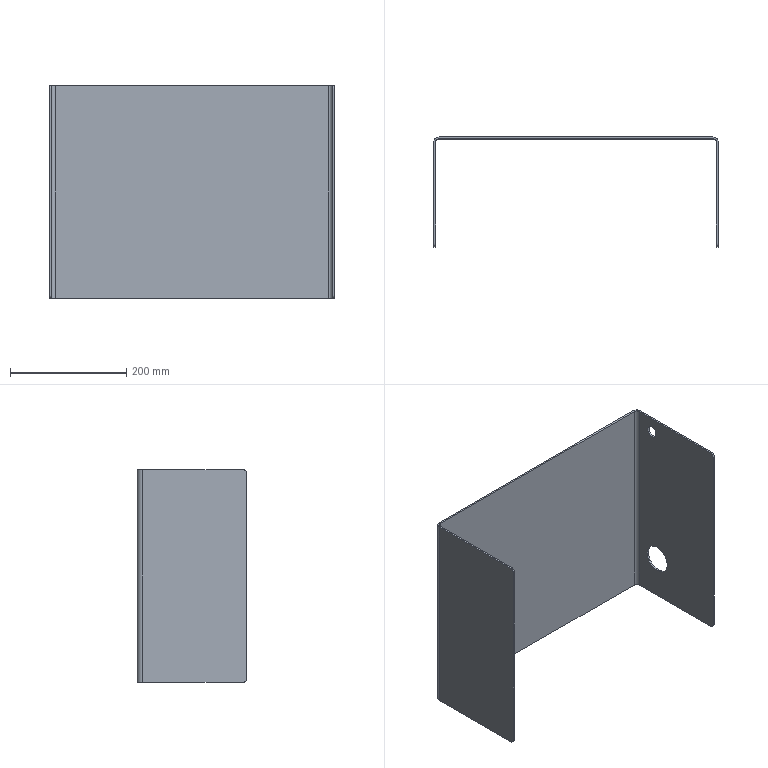Part | SolidWorks | features ICE 3, Cut 1, FlatPattern 1, SMBaseFlange 1, SheetMetal 1 | 1 solid | 30 faces | box 490 x 189 x 366 mm | volume 932829 mm3 | plane 18 | cylinder 12 | commonest cylinder face diameters 12 x6 18 x2 20 x2 48.5 x2
STEP:
#1=CARTESIAN_POINT('',(484.,-37.,349.));
#2=VERTEX_POINT('',#1);
#3=CARTESIAN_POINT('',(484.,-37.,329.));
#4=VERTEX_POINT('',#3);
#5=CARTESIAN_POINT('',(484.,-37.,339.));
#6=DIRECTION('',(1.,0.,0.));
#7=DIRECTION('',(0.,0.,-1.));
#8=AXIS2_PLACEMENT_3D('',#5,#6,#7);
#9=CIRCLE('',#8,10.);
#10=EDGE_CURVE('',#2,#4,#9,.T.);
#11=ORIENTED_EDGE('',*,*,#10,.F.);
#12=CARTESIAN_POINT('',(487.,-37.,349.));
#13=VERTEX_POINT('',#12);
#14=CARTESIAN_POINT('',(477.,-37.,349.));
#15=DIRECTION('',(1.,0.,0.));
#16=VECTOR('',#15,1000.);
#17=LINE('',#14,#16);
#18=EDGE_CURVE('',#2,#13,#17,.T.);
#19=ORIENTED_EDGE('',*,*,#18,.T.);
#20=CARTESIAN_POINT('',(487.,-37.,329.));
#21=VERTEX_POINT('',#20);
#22=CARTESIAN_POINT('',(487.,-37.,339.));
#23=DIRECTION('',(1.,0.,0.));
#24=DIRECTION('',(0.,0.,-1.));
#25=AXIS2_PLACEMENT_3D('',#22,#23,#24);
#26=CIRCLE('',#25,10.);
#27=EDGE_CURVE('',#13,#21,#26,.T.);
#28=ORIENTED_EDGE('',*,*,#27,.T.);
#29=CARTESIAN_POINT('',(477.,-37.,329.));
#30=DIRECTION('',(1.,0.,0.));
#31=VECTOR('',#30,1000.);
#32=LINE('',#29,#31);
#33=EDGE_CURVE('',#4,#21,#32,.T.);
#34=ORIENTED_EDGE('',*,*,#33,.F.);
#35=EDGE_LOOP('',(#11,#19,#28,#34));
#36=FACE_OUTER_BOUND('',#35,.T.);
#37=CARTESIAN_POINT('',(477.,-37.,339.));
#38=DIRECTION('',(1.,0.,0.));
#39=DIRECTION('',(0.,0.,-1.));
#40=AXIS2_PLACEMENT_3D('',#37,#38,#39);
#41=CYLINDRICAL_SURFACE('',#40,10.);
#42=ADVANCED_FACE('',(#36),#41,.F.);
#43=CARTESIAN_POINT('',(484.,-50.,101.25));
#44=VERTEX_POINT('',#43);
#45=CARTESIAN_POINT('',(484.,-50.,52.75));
#46=VERTEX_POINT('',#45);
#47=CARTESIAN_POINT('',(484.,-50.,77.));
#48=DIRECTION('',(1.,0.,0.));
#49=DIRECTION('',(0.,0.,-1.));
#50=AXIS2_PLACEMENT_3D('',#47,#48,#49);
#51=CIRCLE('',#50,24.25);
#52=EDGE_CURVE('',#44,#46,#51,.T.);
#53=ORIENTED_EDGE('',*,*,#52,.F.);
#54=CARTESIAN_POINT('',(487.,-50.,101.25));
#55=VERTEX_POINT('',#54);
#56=CARTESIAN_POINT('',(477.,-50.,101.25));
#57=DIRECTION('',(1.,0.,0.));
#58=VECTOR('',#57,1000.);
#59=LINE('',#56,#58);
#60=EDGE_CURVE('',#44,#55,#59,.T.);
#61=ORIENTED_EDGE('',*,*,#60,.T.);
#62=CARTESIAN_POINT('',(487.,-50.,52.75));
#63=VERTEX_POINT('',#62);
#64=CARTESIAN_POINT('',(487.,-50.,77.));
#65=DIRECTION('',(1.,0.,0.));
#66=DIRECTION('',(0.,0.,-1.));
#67=AXIS2_PLACEMENT_3D('',#64,#65,#66);
#68=CIRCLE('',#67,24.25);
#69=EDGE_CURVE('',#55,#63,#68,.T.);
#70=ORIENTED_EDGE('',*,*,#69,.T.);
#71=CARTESIAN_POINT('',(477.,-50.,52.75));
#72=DIRECTION('',(1.,0.,0.));
#73=VECTOR('',#72,1000.);
#74=LINE('',#71,#73);
#75=EDGE_CURVE('',#46,#63,#74,.T.);
#76=ORIENTED_EDGE('',*,*,#75,.F.);
#77=EDGE_LOOP('',(#53,#61,#70,#76));
#78=FACE_OUTER_BOUND('',#77,.T.);
#79=CARTESIAN_POINT('',(477.,-50.,77.));
#80=DIRECTION('',(1.,0.,0.));
#81=DIRECTION('',(0.,0.,-1.));
#82=AXIS2_PLACEMENT_3D('',#79,#80,#81);
#83=CYLINDRICAL_SURFACE('',#82,24.25);
#84=ADVANCED_FACE('',(#78),#83,.F.);
#85=CARTESIAN_POINT('',(-3.,-180.,0.));
#86=VERTEX_POINT('',#85);
#87=CARTESIAN_POINT('',(-3.,-6.,0.));
#88=VERTEX_POINT('',#87);
#89=CARTESIAN_POINT('',(-3.,0.,0.));
#90=DIRECTION('',(0.,1.,0.));
#91=VECTOR('',#90,1000.);
#92=LINE('',#89,#91);
#93=EDGE_CURVE('',#86,#88,#92,.T.);
#94=ORIENTED_EDGE('',*,*,#93,.F.);
#95=CARTESIAN_POINT('',(-3.,-186.,6.));
#96=VERTEX_POINT('',#95);
#97=CARTESIAN_POINT('',(-3.,-180.,6.));
#98=DIRECTION('',(1.,0.,0.));
#99=DIRECTION('',(0.,-1.,0.));
#100=AXIS2_PLACEMENT_3D('',#97,#98,#99);
#101=CIRCLE('',#100,6.);
#102=EDGE_CURVE('',#96,#86,#101,.T.);
#103=ORIENTED_EDGE('',*,*,#102,.F.);
#104=CARTESIAN_POINT('',(-3.,-186.,360.));
#105=VERTEX_POINT('',#104);
#106=CARTESIAN_POINT('',(-3.,-186.,366.));
#107=DIRECTION('',(0.,0.,1.));
#108=VECTOR('',#107,1000.);
#109=LINE('',#106,#108);
#110=EDGE_CURVE('',#96,#105,#109,.T.);
#111=ORIENTED_EDGE('',*,*,#110,.T.);
#112=CARTESIAN_POINT('',(-3.,-180.,366.));
#113=VERTEX_POINT('',#112);
#114=CARTESIAN_POINT('',(-3.,-180.,360.));
#115=DIRECTION('',(1.,0.,0.));
#116=DIRECTION('',(0.,-1.,0.));
#117=AXIS2_PLACEMENT_3D('',#114,#115,#116);
#118=CIRCLE('',#117,6.);
#119=EDGE_CURVE('',#113,#105,#118,.T.);
#120=ORIENTED_EDGE('',*,*,#119,.F.);
#121=CARTESIAN_POINT('',(-3.,-6.,366.));
#122=VERTEX_POINT('',#121);
#123=CARTESIAN_POINT('',(-3.,0.,366.));
#124=DIRECTION('',(0.,1.,0.));
#125=VECTOR('',#124,1000.);
#126=LINE('',#123,#125);
#127=EDGE_CURVE('',#113,#122,#126,.T.);
#128=ORIENTED_EDGE('',*,*,#127,.T.);
#129=CARTESIAN_POINT('',(-3.,-6.,366.));
#130=DIRECTION('',(0.,0.,-1.));
#131=VECTOR('',#130,1000.);
#132=LINE('',#129,#131);
#133=EDGE_CURVE('',#122,#88,#132,.T.);
#134=ORIENTED_EDGE('',*,*,#133,.T.);
#135=EDGE_LOOP('',(#94,#103,#111,#120,#128,#134));
#136=FACE_OUTER_BOUND('',#135,.T.);
#137=CARTESIAN_POINT('',(-3.,0.,366.));
#138=DIRECTION('',(-1.,0.,0.));
#139=DIRECTION('',(0.,-1.,0.));
#140=AXIS2_PLACEMENT_3D('',#137,#138,#139);
#141=PLANE('',#140);
#142=ADVANCED_FACE('',(#136),#141,.T.);
#143=CARTESIAN_POINT('',(0.,-186.,6.));
#144=VERTEX_POINT('',#143);
#145=CARTESIAN_POINT('',(0.,-180.,0.));
#146=VERTEX_POINT('',#145);
#147=CARTESIAN_POINT('',(0.,-180.,6.));
#148=DIRECTION('',(1.,0.,0.));
#149=DIRECTION('',(0.,-1.,0.));
#150=AXIS2_PLACEMENT_3D('',#147,#148,#149);
#151=CIRCLE('',#150,6.);
#152=EDGE_CURVE('',#144,#146,#151,.T.);
#153=ORIENTED_EDGE('',*,*,#152,.T.);
#154=CARTESIAN_POINT('',(0.,-6.,0.));
#155=VERTEX_POINT('',#154);
#156=CARTESIAN_POINT('',(0.,0.,0.));
#157=DIRECTION('',(0.,1.,0.));
#158=VECTOR('',#157,1000.);
#159=LINE('',#156,#158);
#160=EDGE_CURVE('',#146,#155,#159,.T.);
#161=ORIENTED_EDGE('',*,*,#160,.T.);
#162=CARTESIAN_POINT('',(0.,-6.,366.));
#163=VERTEX_POINT('',#162);
#164=CARTESIAN_POINT('',(0.,-6.,366.));
#165=DIRECTION('',(0.,0.,-1.));
#166=VECTOR('',#165,1000.);
#167=LINE('',#164,#166);
#168=EDGE_CURVE('',#163,#155,#167,.T.);
#169=ORIENTED_EDGE('',*,*,#168,.F.);
#170=CARTESIAN_POINT('',(0.,-180.,366.));
#171=VERTEX_POINT('',#170);
#172=CARTESIAN_POINT('',(0.,0.,366.));
#173=DIRECTION('',(0.,1.,0.));
#174=VECTOR('',#173,1000.);
#175=LINE('',#172,#174);
#176=EDGE_CURVE('',#171,#163,#175,.T.);
#177=ORIENTED_EDGE('',*,*,#176,.F.);
#178=CARTESIAN_POINT('',(0.,-186.,360.));
#179=VERTEX_POINT('',#178);
#180=CARTESIAN_POINT('',(0.,-180.,360.));
#181=DIRECTION('',(1.,0.,0.));
#182=DIRECTION('',(0.,-1.,0.));
#183=AXIS2_PLACEMENT_3D('',#180,#181,#182);
#184=CIRCLE('',#183,6.);
#185=EDGE_CURVE('',#171,#179,#184,.T.);
#186=ORIENTED_EDGE('',*,*,#185,.T.);
#187=CARTESIAN_POINT('',(0.,-186.,366.));
#188=DIRECTION('',(0.,0.,-1.));
#189=VECTOR('',#188,1000.);
#190=LINE('',#187,#189);
#191=EDGE_CURVE('',#179,#144,#190,.T.);
#192=ORIENTED_EDGE('',*,*,#191,.T.);
#193=EDGE_LOOP('',(#153,#161,#169,#177,#186,#192));
#194=FACE_OUTER_BOUND('',#193,.T.);
#195=CARTESIAN_POINT('',(0.,0.,366.));
#196=DIRECTION('',(-1.,0.,0.));
#197=DIRECTION('',(0.,-1.,0.));
#198=AXIS2_PLACEMENT_3D('',#195,#196,#197);
#199=PLANE('',#198);
#200=ADVANCED_FACE('',(#194),#199,.F.);
#201=CARTESIAN_POINT('',(0.,-186.,6.));
#202=DIRECTION('',(-1.,0.,0.));
#203=VECTOR('',#202,1000.);
#204=LINE('',#201,#203);
#205=EDGE_CURVE('',#144,#96,#204,.T.);
#206=ORIENTED_EDGE('',*,*,#205,.F.);
#207=ORIENTED_EDGE('',*,*,#191,.F.);
#208=CARTESIAN_POINT('',(0.,-186.,360.));
#209=DIRECTION('',(-1.,0.,0.));
#210=VECTOR('',#209,1000.);
#211=LINE('',#208,#210);
#212=EDGE_CURVE('',#179,#105,#211,.T.);
#213=ORIENTED_EDGE('',*,*,#212,.T.);
#214=ORIENTED_EDGE('',*,*,#110,.F.);
#215=EDGE_LOOP('',(#206,#207,#213,#214));
#216=FACE_OUTER_BOUND('',#215,.T.);
#217=CARTESIAN_POINT('',(-3.,-186.,366.));
#218=DIRECTION('',(0.,1.,0.));
#219=DIRECTION('',(0.,0.,1.));
#220=AXIS2_PLACEMENT_3D('',#217,#218,#219);
#221=PLANE('',#220);
#222=ADVANCED_FACE('',(#216),#221,.F.);
#223=CARTESIAN_POINT('',(484.,-37.,339.));
#224=DIRECTION('',(1.,0.,0.));
#225=DIRECTION('',(0.,0.,-1.));
#226=AXIS2_PLACEMENT_3D('',#223,#224,#225);
#227=CIRCLE('',#226,10.);
#228=EDGE_CURVE('',#4,#2,#227,.T.);
#229=ORIENTED_EDGE('',*,*,#228,.T.);
#230=ORIENTED_EDGE('',*,*,#10,.T.);
#231=EDGE_LOOP('',(#229,#230));
#232=FACE_BOUND('',#231,.T.);
#233=CARTESIAN_POINT('',(484.,-50.,77.));
#234=DIRECTION('',(1.,0.,0.));
#235=DIRECTION('',(0.,0.,-1.));
#236=AXIS2_PLACEMENT_3D('',#233,#234,#235);
#237=CIRCLE('',#236,24.25);
#238=EDGE_CURVE('',#46,#44,#237,.T.);
#239=ORIENTED_EDGE('',*,*,#238,.T.);
#240=ORIENTED_EDGE('',*,*,#52,.T.);
#241=EDGE_LOOP('',(#239,#240));
#242=FACE_BOUND('',#241,.T.);
#243=CARTESIAN_POINT('',(484.,-186.,360.));
#244=VERTEX_POINT('',#243);
#245=CARTESIAN_POINT('',(484.,-180.,366.));
#246=VERTEX_POINT('',#245);
#247=CARTESIAN_POINT('',(484.,-180.,360.));
#248=DIRECTION('',(-1.,0.,0.));
#249=DIRECTION('',(0.,0.,-1.));
#250=AXIS2_PLACEMENT_3D('',#247,#248,#249);
#251=CIRCLE('',#250,6.);
#252=EDGE_CURVE('',#244,#246,#251,.T.);
#253=ORIENTED_EDGE('',*,*,#252,.T.);
#254=CARTESIAN_POINT('',(484.,-6.,366.));
#255=VERTEX_POINT('',#254);
#256=CARTESIAN_POINT('',(484.,0.,366.));
#257=DIRECTION('',(0.,-1.,0.));
#258=VECTOR('',#257,1000.);
#259=LINE('',#256,#258);
#260=EDGE_CURVE('',#255,#246,#259,.T.);
#261=ORIENTED_EDGE('',*,*,#260,.F.);
#262=CARTESIAN_POINT('',(484.,-6.,0.));
#263=VERTEX_POINT('',#262);
#264=CARTESIAN_POINT('',(484.,-6.,366.));
#265=DIRECTION('',(0.,0.,-1.));
#266=VECTOR('',#265,1000.);
#267=LINE('',#264,#266);
#268=EDGE_CURVE('',#255,#263,#267,.T.);
#269=ORIENTED_EDGE('',*,*,#268,.T.);
#270=CARTESIAN_POINT('',(484.,-180.,0.));
#271=VERTEX_POINT('',#270);
#272=CARTESIAN_POINT('',(484.,0.,0.));
#273=DIRECTION('',(0.,-1.,0.));
#274=VECTOR('',#273,1000.);
#275=LINE('',#272,#274);
#276=EDGE_CURVE('',#263,#271,#275,.T.);
#277=ORIENTED_EDGE('',*,*,#276,.T.);
#278=CARTESIAN_POINT('',(484.,-186.,6.));
#279=VERTEX_POINT('',#278);
#280=CARTESIAN_POINT('',(484.,-180.,6.));
#281=DIRECTION('',(-1.,0.,0.));
#282=DIRECTION('',(0.,0.,-1.));
#283=AXIS2_PLACEMENT_3D('',#280,#281,#282);
#284=CIRCLE('',#283,6.);
#285=EDGE_CURVE('',#271,#279,#284,.T.);
#286=ORIENTED_EDGE('',*,*,#285,.T.);
#287=CARTESIAN_POINT('',(484.,-186.,366.));
#288=DIRECTION('',(0.,0.,1.));
#289=VECTOR('',#288,1000.);
#290=LINE('',#287,#289);
#291=EDGE_CURVE('',#279,#244,#290,.T.);
#292=ORIENTED_EDGE('',*,*,#291,.T.);
#293=EDGE_LOOP('',(#253,#261,#269,#277,#286,#292));
#294=FACE_OUTER_BOUND('',#293,.T.);
#295=CARTESIAN_POINT('',(484.,0.,366.));
#296=DIRECTION('',(1.,0.,0.));
#297=DIRECTION('',(0.,0.,-1.));
#298=AXIS2_PLACEMENT_3D('',#295,#296,#297);
#299=PLANE('',#298);
#300=ADVANCED_FACE('',(#232,#242,#294),#299,.F.);
#301=CARTESIAN_POINT('',(487.,-37.,339.));
#302=DIRECTION('',(1.,0.,0.));
#303=DIRECTION('',(0.,0.,-1.));
#304=AXIS2_PLACEMENT_3D('',#301,#302,#303);
#305=CIRCLE('',#304,10.);
#306=EDGE_CURVE('',#21,#13,#305,.T.);
#307=ORIENTED_EDGE('',*,*,#306,.F.);
#308=ORIENTED_EDGE('',*,*,#27,.F.);
#309=EDGE_LOOP('',(#307,#308));
#310=FACE_BOUND('',#309,.T.);
#311=CARTESIAN_POINT('',(487.,-50.,77.));
#312=DIRECTION('',(1.,0.,0.));
#313=DIRECTION('',(0.,0.,-1.));
#314=AXIS2_PLACEMENT_3D('',#311,#312,#313);
#315=CIRCLE('',#314,24.25);
#316=EDGE_CURVE('',#63,#55,#315,.T.);
#317=ORIENTED_EDGE('',*,*,#316,.F.);
#318=ORIENTED_EDGE('',*,*,#69,.F.);
#319=EDGE_LOOP('',(#317,#318));
#320=FACE_BOUND('',#319,.T.);
#321=CARTESIAN_POINT('',(487.,-6.,366.));
#322=VERTEX_POINT('',#321);
#323=CARTESIAN_POINT('',(487.,-180.,366.));
#324=VERTEX_POINT('',#323);
#325=CARTESIAN_POINT('',(487.,0.,366.));
#326=DIRECTION('',(0.,-1.,0.));
#327=VECTOR('',#326,1000.);
#328=LINE('',#325,#327);
#329=EDGE_CURVE('',#322,#324,#328,.T.);
#330=ORIENTED_EDGE('',*,*,#329,.T.);
#331=CARTESIAN_POINT('',(487.,-186.,360.));
#332=VERTEX_POINT('',#331);
#333=CARTESIAN_POINT('',(487.,-180.,360.));
#334=DIRECTION('',(-1.,0.,0.));
#335=DIRECTION('',(0.,0.,-1.));
#336=AXIS2_PLACEMENT_3D('',#333,#334,#335);
#337=CIRCLE('',#336,6.);
#338=EDGE_CURVE('',#332,#324,#337,.T.);
#339=ORIENTED_EDGE('',*,*,#338,.F.);
#340=CARTESIAN_POINT('',(487.,-186.,6.));
#341=VERTEX_POINT('',#340);
#342=CARTESIAN_POINT('',(487.,-186.,366.));
#343=DIRECTION('',(0.,0.,1.));
#344=VECTOR('',#343,1000.);
#345=LINE('',#342,#344);
#346=EDGE_CURVE('',#341,#332,#345,.T.);
#347=ORIENTED_EDGE('',*,*,#346,.F.);
#348=CARTESIAN_POINT('',(487.,-180.,0.));
#349=VERTEX_POINT('',#348);
#350=CARTESIAN_POINT('',(487.,-180.,6.));
#351=DIRECTION('',(-1.,0.,0.));
#352=DIRECTION('',(0.,0.,-1.));
#353=AXIS2_PLACEMENT_3D('',#350,#351,#352);
#354=CIRCLE('',#353,6.);
#355=EDGE_CURVE('',#349,#341,#354,.T.);
#356=ORIENTED_EDGE('',*,*,#355,.F.);
#357=CARTESIAN_POINT('',(487.,-6.,0.));
#358=VERTEX_POINT('',#357);
#359=CARTESIAN_POINT('',(487.,0.,0.));
#360=DIRECTION('',(0.,-1.,0.));
#361=VECTOR('',#360,1000.);
#362=LINE('',#359,#361);
#363=EDGE_CURVE('',#358,#349,#362,.T.);
#364=ORIENTED_EDGE('',*,*,#363,.F.);
#365=CARTESIAN_POINT('',(487.,-6.,366.));
#366=DIRECTION('',(0.,0.,-1.));
#367=VECTOR('',#366,1000.);
#368=LINE('',#365,#367);
#369=EDGE_CURVE('',#322,#358,#368,.T.);
#370=ORIENTED_EDGE('',*,*,#369,.F.);
#371=EDGE_LOOP('',(#330,#339,#347,#356,#364,#370));
#372=FACE_OUTER_BOUND('',#371,.T.);
#373=CARTESIAN_POINT('',(487.,0.,366.));
#374=DIRECTION('',(1.,0.,0.));
#375=DIRECTION('',(0.,0.,-1.));
#376=AXIS2_PLACEMENT_3D('',#373,#374,#375);
#377=PLANE('',#376);
#378=ADVANCED_FACE('',(#310,#320,#372),#377,.T.);
#379=ORIENTED_EDGE('',*,*,#260,.T.);
#380=CARTESIAN_POINT('',(484.,-180.,366.));
#381=DIRECTION('',(1.,0.,0.));
#382=VECTOR('',#381,1000.);
#383=LINE('',#380,#382);
#384=EDGE_CURVE('',#246,#324,#383,.T.);
#385=ORIENTED_EDGE('',*,*,#384,.T.);
#386=ORIENTED_EDGE('',*,*,#329,.F.);
#387=CARTESIAN_POINT('',(487.,-6.,366.));
#388=DIRECTION('',(-1.,0.,0.));
#389=VECTOR('',#388,1000.);
#390=LINE('',#387,#389);
#391=EDGE_CURVE('',#322,#255,#390,.T.);
#392=ORIENTED_EDGE('',*,*,#391,.T.);
#393=EDGE_LOOP('',(#379,#385,#386,#392));
#394=FACE_OUTER_BOUND('',#393,.T.);
#395=CARTESIAN_POINT('',(478.,-6.,366.));
#396=DIRECTION('',(0.,0.,1.));
#397=DIRECTION('',(1.,0.,0.));
#398=AXIS2_PLACEMENT_3D('',#395,#396,#397);
#399=PLANE('',#398);
#400=ADVANCED_FACE('',(#394),#399,.T.);
#401=CARTESIAN_POINT('',(484.,-186.,360.));
#402=DIRECTION('',(1.,0.,0.));
#403=VECTOR('',#402,1000.);
#404=LINE('',#401,#403);
#405=EDGE_CURVE('',#244,#332,#404,.T.);
#406=ORIENTED_EDGE('',*,*,#405,.F.);
#407=ORIENTED_EDGE('',*,*,#291,.F.);
#408=CARTESIAN_POINT('',(484.,-186.,6.));
#409=DIRECTION('',(1.,0.,0.));
#410=VECTOR('',#409,1000.);
#411=LINE('',#408,#410);
#412=EDGE_CURVE('',#279,#341,#411,.T.);
#413=ORIENTED_EDGE('',*,*,#412,.T.);
#414=ORIENTED_EDGE('',*,*,#346,.T.);
#415=EDGE_LOOP('',(#406,#407,#413,#414));
#416=FACE_OUTER_BOUND('',#415,.T.);
#417=CARTESIAN_POINT('',(-3.,-186.,366.));
#418=DIRECTION('',(0.,1.,0.));
#419=DIRECTION('',(0.,0.,1.));
#420=AXIS2_PLACEMENT_3D('',#417,#418,#419);
#421=PLANE('',#420);
#422=ADVANCED_FACE('',(#416),#421,.F.);
#423=CARTESIAN_POINT('',(0.,-6.,366.));
#424=DIRECTION('',(-1.,0.,0.));
#425=VECTOR('',#424,1000.);
#426=LINE('',#423,#425);
#427=EDGE_CURVE('',#163,#122,#426,.T.);
#428=ORIENTED_EDGE('',*,*,#427,.F.);
#429=CARTESIAN_POINT('',(6.,0.,366.));
#430=VERTEX_POINT('',#429);
#431=CARTESIAN_POINT('',(6.,-6.,366.));
#432=DIRECTION('',(0.,0.,-1.));
#433=DIRECTION('',(1.,0.,0.));
#434=AXIS2_PLACEMENT_3D('',#431,#432,#433);
#435=CIRCLE('',#434,6.);
#436=EDGE_CURVE('',#163,#430,#435,.T.);
#437=ORIENTED_EDGE('',*,*,#436,.T.);
#438=CARTESIAN_POINT('',(6.,3.,366.));
#439=VERTEX_POINT('',#438);
#440=CARTESIAN_POINT('',(6.,3.,366.));
#441=DIRECTION('',(0.,-1.,0.));
#442=VECTOR('',#441,1000.);
#443=LINE('',#440,#442);
#444=EDGE_CURVE('',#439,#430,#443,.T.);
#445=ORIENTED_EDGE('',*,*,#444,.F.);
#446=CARTESIAN_POINT('',(6.,-6.,366.));
#447=DIRECTION('',(0.,0.,-1.));
#448=DIRECTION('',(1.,0.,0.));
#449=AXIS2_PLACEMENT_3D('',#446,#447,#448);
#450=CIRCLE('',#449,9.);
#451=EDGE_CURVE('',#122,#439,#450,.T.);
#452=ORIENTED_EDGE('',*,*,#451,.F.);
#453=EDGE_LOOP('',(#428,#437,#445,#452));
#454=FACE_OUTER_BOUND('',#453,.T.);
#455=CARTESIAN_POINT('',(0.,-6.,366.));
#456=DIRECTION('',(0.,0.,1.));
#457=DIRECTION('',(1.,0.,0.));
#458=AXIS2_PLACEMENT_3D('',#455,#456,#457);
#459=PLANE('',#458);
#460=ADVANCED_FACE('',(#454),#459,.T.);
#461=CARTESIAN_POINT('',(0.,-180.,366.));
#462=DIRECTION('',(-1.,0.,0.));
#463=VECTOR('',#462,1000.);
#464=LINE('',#461,#463);
#465=EDGE_CURVE('',#171,#113,#464,.T.);
#466=ORIENTED_EDGE('',*,*,#465,.F.);
#467=ORIENTED_EDGE('',*,*,#176,.T.);
#468=ORIENTED_EDGE('',*,*,#427,.T.);
#469=ORIENTED_EDGE('',*,*,#127,.F.);
#470=EDGE_LOOP('',(#466,#467,#468,#469));
#471=FACE_OUTER_BOUND('',#470,.T.);
#472=CARTESIAN_POINT('',(6.,3.,366.));
#473=DIRECTION('',(0.,0.,1.));
#474=DIRECTION('',(1.,0.,0.));
#475=AXIS2_PLACEMENT_3D('',#472,#473,#474);
#476=PLANE('',#475);
#477=ADVANCED_FACE('',(#471),#476,.T.);
#478=CARTESIAN_POINT('',(6.,0.,0.));
#479=VERTEX_POINT('',#478);
#480=CARTESIAN_POINT('',(6.,3.,0.));
#481=VERTEX_POINT('',#480);
#482=CARTESIAN_POINT('',(6.,0.,0.));
#483=DIRECTION('',(0.,1.,0.));
#484=VECTOR('',#483,1000.);
#485=LINE('',#482,#484);
#486=EDGE_CURVE('',#479,#481,#485,.T.);
#487=ORIENTED_EDGE('',*,*,#486,.F.);
#488=CARTESIAN_POINT('',(6.,-6.,0.));
#489=DIRECTION('',(0.,0.,-1.));
#490=DIRECTION('',(1.,0.,0.));
#491=AXIS2_PLACEMENT_3D('',#488,#489,#490);
#492=CIRCLE('',#491,6.);
#493=EDGE_CURVE('',#155,#479,#492,.T.);
#494=ORIENTED_EDGE('',*,*,#493,.F.);
#495=CARTESIAN_POINT('',(-3.,-6.,0.));
#496=DIRECTION('',(1.,0.,0.));
#497=VECTOR('',#496,1000.);
#498=LINE('',#495,#497);
#499=EDGE_CURVE('',#88,#155,#498,.T.);
#500=ORIENTED_EDGE('',*,*,#499,.F.);
#501=CARTESIAN_POINT('',(6.,-6.,0.));
#502=DIRECTION('',(0.,0.,-1.));
#503=DIRECTION('',(1.,0.,0.));
#504=AXIS2_PLACEMENT_3D('',#501,#502,#503);
#505=CIRCLE('',#504,9.);
#506=EDGE_CURVE('',#88,#481,#505,.T.);
#507=ORIENTED_EDGE('',*,*,#506,.T.);
#508=EDGE_LOOP('',(#487,#494,#500,#507));
#509=FACE_OUTER_BOUND('',#508,.T.);
#510=CARTESIAN_POINT('',(6.,0.,0.));
#511=DIRECTION('',(0.,0.,-1.));
#512=DIRECTION('',(-1.,0.,0.));
#513=AXIS2_PLACEMENT_3D('',#510,#511,#512);
#514=PLANE('',#513);
#515=ADVANCED_FACE('',(#509),#514,.T.);
#516=CARTESIAN_POINT('',(478.,0.,0.));
#517=VERTEX_POINT('',#516);
#518=CARTESIAN_POINT('',(0.,0.,0.));
#519=DIRECTION('',(1.,0.,0.));
#520=VECTOR('',#519,1000.);
#521=LINE('',#518,#520);
#522=EDGE_CURVE('',#479,#517,#521,.T.);
#523=ORIENTED_EDGE('',*,*,#522,.F.);
#524=ORIENTED_EDGE('',*,*,#486,.T.);
#525=CARTESIAN_POINT('',(478.,3.,0.));
#526=VERTEX_POINT('',#525);
#527=CARTESIAN_POINT('',(0.,3.,0.));
#528=DIRECTION('',(1.,0.,0.));
#529=VECTOR('',#528,1000.);
#530=LINE('',#527,#529);
#531=EDGE_CURVE('',#481,#526,#530,.T.);
#532=ORIENTED_EDGE('',*,*,#531,.T.);
#533=CARTESIAN_POINT('',(478.,3.,0.));
#534=DIRECTION('',(0.,-1.,0.));
#535=VECTOR('',#534,1000.);
#536=LINE('',#533,#535);
#537=EDGE_CURVE('',#526,#517,#536,.T.);
#538=ORIENTED_EDGE('',*,*,#537,.T.);
#539=EDGE_LOOP('',(#523,#524,#532,#538));
#540=FACE_OUTER_BOUND('',#539,.T.);
#541=CARTESIAN_POINT('',(-3.,-6.,0.));
#542=DIRECTION('',(0.,0.,-1.));
#543=DIRECTION('',(-1.,0.,0.));
#544=AXIS2_PLACEMENT_3D('',#541,#542,#543);
#545=PLANE('',#544);
#546=ADVANCED_FACE('',(#540),#545,.T.);
#547=CARTESIAN_POINT('',(478.,0.,366.));
#548=VERTEX_POINT('',#547);
#549=CARTESIAN_POINT('',(478.,3.,366.));
#550=VERTEX_POINT('',#549);
#551=CARTESIAN_POINT('',(478.,0.,366.));
#552=DIRECTION('',(0.,1.,0.));
#553=VECTOR('',#552,1000.);
#554=LINE('',#551,#553);
#555=EDGE_CURVE('',#548,#550,#554,.T.);
#556=ORIENTED_EDGE('',*,*,#555,.F.);
#557=CARTESIAN_POINT('',(478.,-6.,366.));
#558=DIRECTION('',(0.,0.,-1.));
#559=DIRECTION('',(1.,0.,0.));
#560=AXIS2_PLACEMENT_3D('',#557,#558,#559);
#561=CIRCLE('',#560,6.);
#562=EDGE_CURVE('',#548,#255,#561,.T.);
#563=ORIENTED_EDGE('',*,*,#562,.T.);
#564=ORIENTED_EDGE('',*,*,#391,.F.);
#565=CARTESIAN_POINT('',(478.,-6.,366.));
#566=DIRECTION('',(0.,0.,-1.));
#567=DIRECTION('',(1.,0.,0.));
#568=AXIS2_PLACEMENT_3D('',#565,#566,#567);
#569=CIRCLE('',#568,9.);
#570=EDGE_CURVE('',#550,#322,#569,.T.);
#571=ORIENTED_EDGE('',*,*,#570,.F.);
#572=EDGE_LOOP('',(#556,#563,#564,#571));
#573=FACE_OUTER_BOUND('',#572,.T.);
#574=CARTESIAN_POINT('',(478.,0.,366.));
#575=DIRECTION('',(0.,0.,1.));
#576=DIRECTION('',(1.,0.,0.));
#577=AXIS2_PLACEMENT_3D('',#574,#575,#576);
#578=PLANE('',#577);
#579=ADVANCED_FACE('',(#573),#578,.T.);
#580=CARTESIAN_POINT('',(0.,0.,366.));
#581=DIRECTION('',(1.,0.,0.));
#582=VECTOR('',#581,1000.);
#583=LINE('',#580,#582);
#584=EDGE_CURVE('',#430,#548,#583,.T.);
#585=ORIENTED_EDGE('',*,*,#584,.T.);
#586=ORIENTED_EDGE('',*,*,#555,.T.);
#587=CARTESIAN_POINT('',(0.,3.,366.));
#588=DIRECTION('',(1.,0.,0.));
#589=VECTOR('',#588,1000.);
#590=LINE('',#587,#589);
#591=EDGE_CURVE('',#439,#550,#590,.T.);
#592=ORIENTED_EDGE('',*,*,#591,.F.);
#593=ORIENTED_EDGE('',*,*,#444,.T.);
#594=EDGE_LOOP('',(#585,#586,#592,#593));
#595=FACE_OUTER_BOUND('',#594,.T.);
#596=CARTESIAN_POINT('',(487.,-6.,366.));
#597=DIRECTION('',(0.,0.,1.));
#598=DIRECTION('',(1.,0.,0.));
#599=AXIS2_PLACEMENT_3D('',#596,#597,#598);
#600=PLANE('',#599);
#601=ADVANCED_FACE('',(#595),#600,.T.);
#602=CARTESIAN_POINT('',(484.,-6.,0.));
#603=DIRECTION('',(1.,0.,0.));
#604=VECTOR('',#603,1000.);
#605=LINE('',#602,#604);
#606=EDGE_CURVE('',#263,#358,#605,.T.);
#607=ORIENTED_EDGE('',*,*,#606,.F.);
#608=CARTESIAN_POINT('',(478.,-6.,0.));
#609=DIRECTION('',(0.,0.,-1.));
#610=DIRECTION('',(1.,0.,0.));
#611=AXIS2_PLACEMENT_3D('',#608,#609,#610);
#612=CIRCLE('',#611,6.);
#613=EDGE_CURVE('',#517,#263,#612,.T.);
#614=ORIENTED_EDGE('',*,*,#613,.F.);
#615=ORIENTED_EDGE('',*,*,#537,.F.);
#616=CARTESIAN_POINT('',(478.,-6.,0.));
#617=DIRECTION('',(0.,0.,-1.));
#618=DIRECTION('',(1.,0.,0.));
#619=AXIS2_PLACEMENT_3D('',#616,#617,#618);
#620=CIRCLE('',#619,9.);
#621=EDGE_CURVE('',#526,#358,#620,.T.);
#622=ORIENTED_EDGE('',*,*,#621,.T.);
#623=EDGE_LOOP('',(#607,#614,#615,#622));
#624=FACE_OUTER_BOUND('',#623,.T.);
#625=CARTESIAN_POINT('',(484.,-6.,0.));
#626=DIRECTION('',(0.,0.,-1.));
#627=DIRECTION('',(-1.,0.,0.));
#628=AXIS2_PLACEMENT_3D('',#625,#626,#627);
#629=PLANE('',#628);
#630=ADVANCED_FACE('',(#624),#629,.T.);
#631=CARTESIAN_POINT('',(484.,-180.,0.));
#632=DIRECTION('',(1.,0.,0.));
#633=VECTOR('',#632,1000.);
#634=LINE('',#631,#633);
#635=EDGE_CURVE('',#271,#349,#634,.T.);
#636=ORIENTED_EDGE('',*,*,#635,.F.);
#637=ORIENTED_EDGE('',*,*,#276,.F.);
#638=ORIENTED_EDGE('',*,*,#606,.T.);
#639=ORIENTED_EDGE('',*,*,#363,.T.);
#640=EDGE_LOOP('',(#636,#637,#638,#639));
#641=FACE_OUTER_BOUND('',#640,.T.);
#642=CARTESIAN_POINT('',(478.,3.,0.));
#643=DIRECTION('',(0.,0.,-1.));
#644=DIRECTION('',(-1.,0.,0.));
#645=AXIS2_PLACEMENT_3D('',#642,#643,#644);
#646=PLANE('',#645);
#647=ADVANCED_FACE('',(#641),#646,.T.);
#648=ORIENTED_EDGE('',*,*,#621,.F.);
#649=CARTESIAN_POINT('',(478.,3.,366.));
#650=DIRECTION('',(0.,0.,-1.));
#651=VECTOR('',#650,1000.);
#652=LINE('',#649,#651);
#653=EDGE_CURVE('',#550,#526,#652,.T.);
#654=ORIENTED_EDGE('',*,*,#653,.F.);
#655=ORIENTED_EDGE('',*,*,#570,.T.);
#656=ORIENTED_EDGE('',*,*,#369,.T.);
#657=EDGE_LOOP('',(#648,#654,#655,#656));
#658=FACE_OUTER_BOUND('',#657,.T.);
#659=CARTESIAN_POINT('',(478.,-6.,366.));
#660=DIRECTION('',(0.,0.,-1.));
#661=DIRECTION('',(-1.,0.,0.));
#662=AXIS2_PLACEMENT_3D('',#659,#660,#661);
#663=CYLINDRICAL_SURFACE('',#662,9.);
#664=ADVANCED_FACE('',(#658),#663,.T.);
#665=ORIENTED_EDGE('',*,*,#531,.F.);
#666=CARTESIAN_POINT('',(6.,3.,366.));
#667=DIRECTION('',(0.,0.,-1.));
#668=VECTOR('',#667,1000.);
#669=LINE('',#666,#668);
#670=EDGE_CURVE('',#439,#481,#669,.T.);
#671=ORIENTED_EDGE('',*,*,#670,.F.);
#672=ORIENTED_EDGE('',*,*,#591,.T.);
#673=ORIENTED_EDGE('',*,*,#653,.T.);
#674=EDGE_LOOP('',(#665,#671,#672,#673));
#675=FACE_OUTER_BOUND('',#674,.T.);
#676=CARTESIAN_POINT('',(0.,3.,366.));
#677=DIRECTION('',(0.,1.,0.));
#678=DIRECTION('',(0.,0.,1.));
#679=AXIS2_PLACEMENT_3D('',#676,#677,#678);
#680=PLANE('',#679);
#681=ADVANCED_FACE('',(#675),#680,.T.);
#682=ORIENTED_EDGE('',*,*,#506,.F.);
#683=ORIENTED_EDGE('',*,*,#133,.F.);
#684=ORIENTED_EDGE('',*,*,#451,.T.);
#685=ORIENTED_EDGE('',*,*,#670,.T.);
#686=EDGE_LOOP('',(#682,#683,#684,#685));
#687=FACE_OUTER_BOUND('',#686,.T.);
#688=CARTESIAN_POINT('',(6.,-6.,366.));
#689=DIRECTION('',(0.,0.,-1.));
#690=DIRECTION('',(-1.,0.,0.));
#691=AXIS2_PLACEMENT_3D('',#688,#689,#690);
#692=CYLINDRICAL_SURFACE('',#691,9.);
#693=ADVANCED_FACE('',(#687),#692,.T.);
#694=ORIENTED_EDGE('',*,*,#493,.T.);
#695=CARTESIAN_POINT('',(6.,0.,366.));
#696=DIRECTION('',(0.,0.,-1.));
#697=VECTOR('',#696,1000.);
#698=LINE('',#695,#697);
#699=EDGE_CURVE('',#430,#479,#698,.T.);
#700=ORIENTED_EDGE('',*,*,#699,.F.);
#701=ORIENTED_EDGE('',*,*,#436,.F.);
#702=ORIENTED_EDGE('',*,*,#168,.T.);
#703=EDGE_LOOP('',(#694,#700,#701,#702));
#704=FACE_OUTER_BOUND('',#703,.T.);
#705=CARTESIAN_POINT('',(6.,-6.,366.));
#706=DIRECTION('',(0.,0.,-1.));
#707=DIRECTION('',(-1.,0.,0.));
#708=AXIS2_PLACEMENT_3D('',#705,#706,#707);
#709=CYLINDRICAL_SURFACE('',#708,6.);
#710=ADVANCED_FACE('',(#704),#709,.F.);
#711=ORIENTED_EDGE('',*,*,#522,.T.);
#712=CARTESIAN_POINT('',(478.,0.,366.));
#713=DIRECTION('',(0.,0.,-1.));
#714=VECTOR('',#713,1000.);
#715=LINE('',#712,#714);
#716=EDGE_CURVE('',#548,#517,#715,.T.);
#717=ORIENTED_EDGE('',*,*,#716,.F.);
#718=ORIENTED_EDGE('',*,*,#584,.F.);
#719=ORIENTED_EDGE('',*,*,#699,.T.);
#720=EDGE_LOOP('',(#711,#717,#718,#719));
#721=FACE_OUTER_BOUND('',#720,.T.);
#722=CARTESIAN_POINT('',(0.,0.,366.));
#723=DIRECTION('',(0.,1.,0.));
#724=DIRECTION('',(0.,0.,1.));
#725=AXIS2_PLACEMENT_3D('',#722,#723,#724);
#726=PLANE('',#725);
#727=ADVANCED_FACE('',(#721),#726,.F.);
#728=ORIENTED_EDGE('',*,*,#613,.T.);
#729=ORIENTED_EDGE('',*,*,#268,.F.);
#730=ORIENTED_EDGE('',*,*,#562,.F.);
#731=ORIENTED_EDGE('',*,*,#716,.T.);
#732=EDGE_LOOP('',(#728,#729,#730,#731));
#733=FACE_OUTER_BOUND('',#732,.T.);
#734=CARTESIAN_POINT('',(478.,-6.,366.));
#735=DIRECTION('',(0.,0.,-1.));
#736=DIRECTION('',(-1.,0.,0.));
#737=AXIS2_PLACEMENT_3D('',#734,#735,#736);
#738=CYLINDRICAL_SURFACE('',#737,6.);
#739=ADVANCED_FACE('',(#733),#738,.F.);
#740=ORIENTED_EDGE('',*,*,#160,.F.);
#741=CARTESIAN_POINT('',(0.,-180.,0.));
#742=DIRECTION('',(-1.,0.,0.));
#743=VECTOR('',#742,1000.);
#744=LINE('',#741,#743);
#745=EDGE_CURVE('',#146,#86,#744,.T.);
#746=ORIENTED_EDGE('',*,*,#745,.T.);
#747=ORIENTED_EDGE('',*,*,#93,.T.);
#748=ORIENTED_EDGE('',*,*,#499,.T.);
#749=EDGE_LOOP('',(#740,#746,#747,#748));
#750=FACE_OUTER_BOUND('',#749,.T.);
#751=CARTESIAN_POINT('',(478.,-6.,0.));
#752=DIRECTION('',(0.,0.,1.));
#753=DIRECTION('',(1.,0.,0.));
#754=AXIS2_PLACEMENT_3D('',#751,#752,#753);
#755=PLANE('',#754);
#756=ADVANCED_FACE('',(#750),#755,.F.);
#757=ORIENTED_EDGE('',*,*,#212,.F.);
#758=ORIENTED_EDGE('',*,*,#185,.F.);
#759=ORIENTED_EDGE('',*,*,#465,.T.);
#760=ORIENTED_EDGE('',*,*,#119,.T.);
#761=EDGE_LOOP('',(#757,#758,#759,#760));
#762=FACE_OUTER_BOUND('',#761,.T.);
#763=CARTESIAN_POINT('',(0.,-180.,360.));
#764=DIRECTION('',(-1.,0.,0.));
#765=DIRECTION('',(0.,-1.,0.));
#766=AXIS2_PLACEMENT_3D('',#763,#764,#765);
#767=CYLINDRICAL_SURFACE('',#766,6.);
#768=ADVANCED_FACE('',(#762),#767,.T.);
#769=ORIENTED_EDGE('',*,*,#412,.F.);
#770=ORIENTED_EDGE('',*,*,#285,.F.);
#771=ORIENTED_EDGE('',*,*,#635,.T.);
#772=ORIENTED_EDGE('',*,*,#355,.T.);
#773=EDGE_LOOP('',(#769,#770,#771,#772));
#774=FACE_OUTER_BOUND('',#773,.T.);
#775=CARTESIAN_POINT('',(484.,-180.,6.));
#776=DIRECTION('',(1.,0.,0.));
#777=DIRECTION('',(0.,0.,-1.));
#778=AXIS2_PLACEMENT_3D('',#775,#776,#777);
#779=CYLINDRICAL_SURFACE('',#778,6.);
#780=ADVANCED_FACE('',(#774),#779,.T.);
#781=ORIENTED_EDGE('',*,*,#384,.F.);
#782=ORIENTED_EDGE('',*,*,#252,.F.);
#783=ORIENTED_EDGE('',*,*,#405,.T.);
#784=ORIENTED_EDGE('',*,*,#338,.T.);
#785=EDGE_LOOP('',(#781,#782,#783,#784));
#786=FACE_OUTER_BOUND('',#785,.T.);
#787=CARTESIAN_POINT('',(484.,-180.,360.));
#788=DIRECTION('',(1.,0.,0.));
#789=DIRECTION('',(0.,0.,-1.));
#790=AXIS2_PLACEMENT_3D('',#787,#788,#789);
#791=CYLINDRICAL_SURFACE('',#790,6.);
#792=ADVANCED_FACE('',(#786),#791,.T.);
#793=ORIENTED_EDGE('',*,*,#745,.F.);
#794=ORIENTED_EDGE('',*,*,#152,.F.);
#795=ORIENTED_EDGE('',*,*,#205,.T.);
#796=ORIENTED_EDGE('',*,*,#102,.T.);
#797=EDGE_LOOP('',(#793,#794,#795,#796));
#798=FACE_OUTER_BOUND('',#797,.T.);
#799=CARTESIAN_POINT('',(0.,-180.,6.));
#800=DIRECTION('',(-1.,0.,0.));
#801=DIRECTION('',(0.,-1.,0.));
#802=AXIS2_PLACEMENT_3D('',#799,#800,#801);
#803=CYLINDRICAL_SURFACE('',#802,6.);
#804=ADVANCED_FACE('',(#798),#803,.T.);
#805=ORIENTED_EDGE('',*,*,#60,.F.);
#806=ORIENTED_EDGE('',*,*,#238,.F.);
#807=ORIENTED_EDGE('',*,*,#75,.T.);
#808=ORIENTED_EDGE('',*,*,#316,.T.);
#809=EDGE_LOOP('',(#805,#806,#807,#808));
#810=FACE_OUTER_BOUND('',#809,.T.);
#811=CARTESIAN_POINT('',(477.,-50.,77.));
#812=DIRECTION('',(1.,0.,0.));
#813=DIRECTION('',(0.,0.,-1.));
#814=AXIS2_PLACEMENT_3D('',#811,#812,#813);
#815=CYLINDRICAL_SURFACE('',#814,24.25);
#816=ADVANCED_FACE('',(#810),#815,.F.);
#817=ORIENTED_EDGE('',*,*,#18,.F.);
#818=ORIENTED_EDGE('',*,*,#228,.F.);
#819=ORIENTED_EDGE('',*,*,#33,.T.);
#820=ORIENTED_EDGE('',*,*,#306,.T.);
#821=EDGE_LOOP('',(#817,#818,#819,#820));
#822=FACE_OUTER_BOUND('',#821,.T.);
#823=CARTESIAN_POINT('',(477.,-37.,339.));
#824=DIRECTION('',(1.,0.,0.));
#825=DIRECTION('',(0.,0.,-1.));
#826=AXIS2_PLACEMENT_3D('',#823,#824,#825);
#827=CYLINDRICAL_SURFACE('',#826,10.);
#828=ADVANCED_FACE('',(#822),#827,.F.);
#829=CLOSED_SHELL('',(#42,#84,#142,#200,#222,#300,#378,#400,#422,#460,#477,#515,#546,#579,#601,#630,#647,#664,#681,#693,#710,#727,#739,#756,#768,#780,#792,#804,#816,#828));
#830=MANIFOLD_SOLID_BREP('',#829);
#831=CARTESIAN_POINT('',(0.,0.,0.));
#832=DIRECTION('',(0.,0.,1.));
#833=DIRECTION('',(1.,0.,0.));
#834=AXIS2_PLACEMENT_3D('',#831,#832,#833);
#835=(LENGTH_UNIT()NAMED_UNIT(*)SI_UNIT(.MILLI.,.METRE.));
#836=UNCERTAINTY_MEASURE_WITH_UNIT(LENGTH_MEASURE(0.00001),#835,'','');
#837=(NAMED_UNIT(*)PLANE_ANGLE_UNIT()SI_UNIT($,.RADIAN.));
#838=(NAMED_UNIT(*)SI_UNIT($,.STERADIAN.)SOLID_ANGLE_UNIT());
#839=(GEOMETRIC_REPRESENTATION_CONTEXT(3)GLOBAL_UNCERTAINTY_ASSIGNED_CONTEXT((#836))GLOBAL_UNIT_ASSIGNED_CONTEXT((#835,#837,#838))REPRESENTATION_CONTEXT('',''));
#840=ADVANCED_BREP_SHAPE_REPRESENTATION('',(#830,#834),#839);